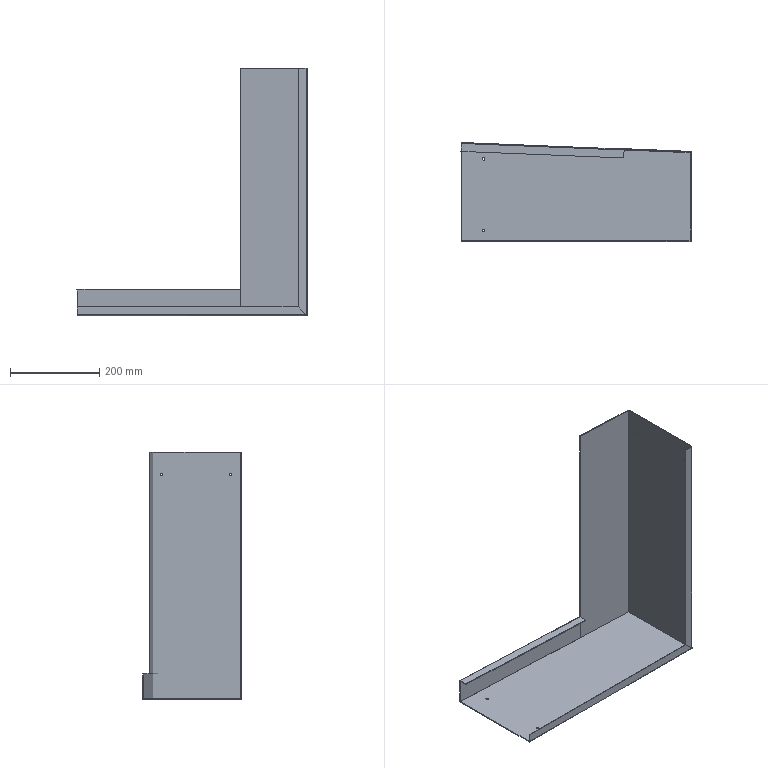Part | STEP file | TS-S18 | 1 solid | 68 faces | box 515.803 x 221.885 x 555 mm | volume 694514 mm3 | plane 45 | cylinder 20 | spline 3 | commonest cylinder face diameters 5.4 x8 0.4 x6 4.4 x6